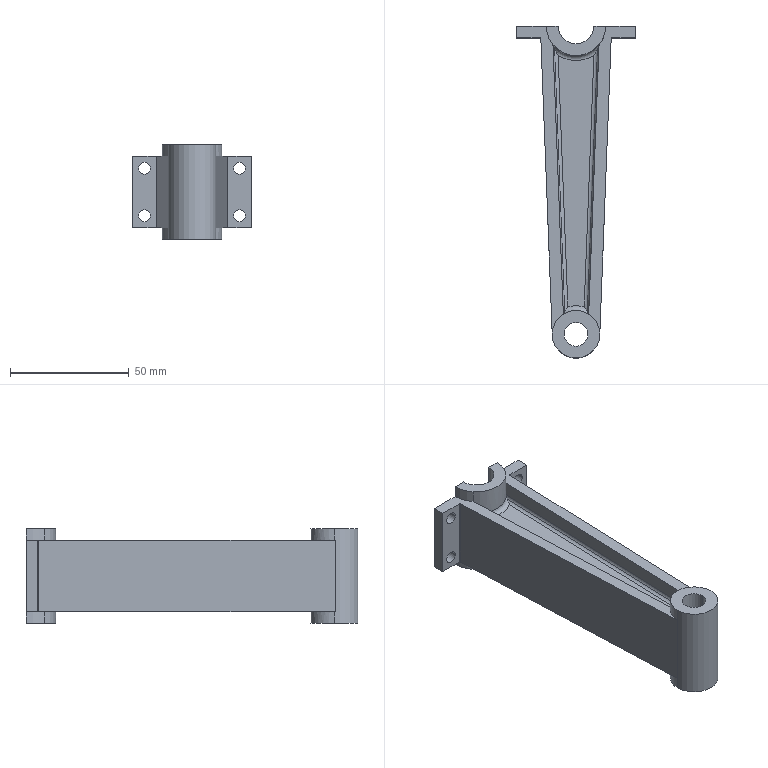Part | SolidWorks | features BaseBody 1 | 1 solid | 56 faces | box 50 x 139.8 x 40 mm | volume 78010 mm3 | cylinder 30 | plane 22 | torus 4 | commonest cylinder face diameters 4 x8 5 x8 0.5 x4 25 x4 20 x3 10 x2